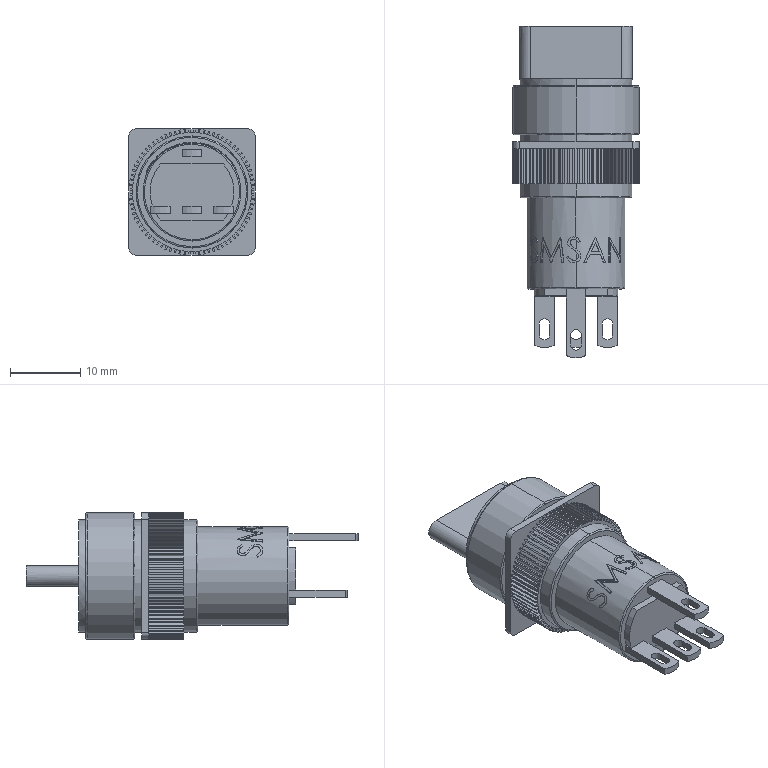Part | STEP file | Round selector switch[GQ115-C-11XA]_GQ115-C-11XA | 1 solid | 489 faces | box 18 x 47.347 x 18 mm | volume 5818 mm3 | plane 304 | cylinder 127 | spline 58 | commonest cylinder face diameters 18 x82 1.5 x8 14.2 x8 14 x7 2 x6 16 x6